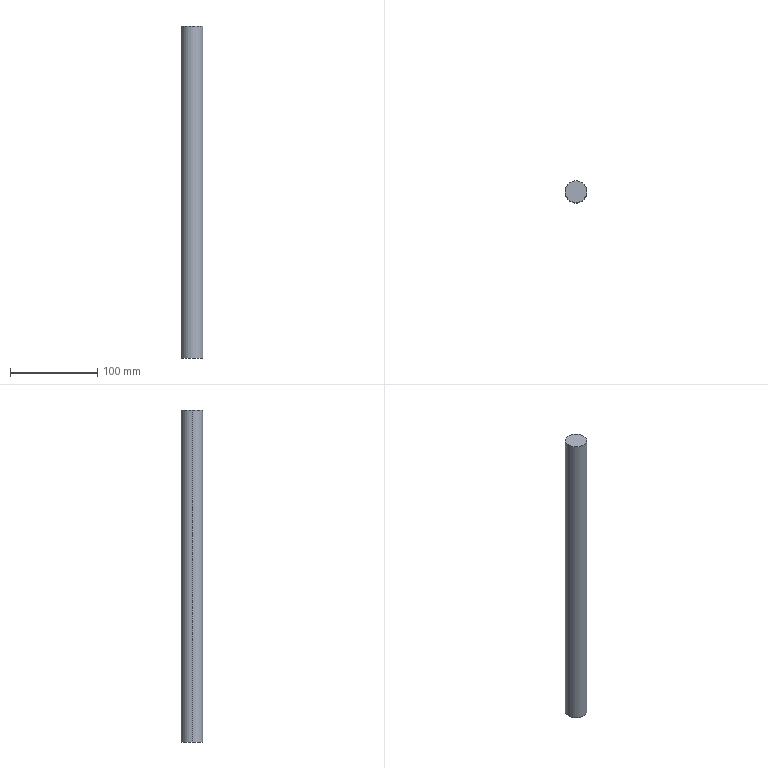Part | STEP file | 1 solid | 4 faces | box 25 x 25 x 380 mm | volume 186532 mm3 | cylinder 2 | plane 2 | commonest cylinder face diameters 25 x2
STEP:
#1=CARTESIAN_POINT('',(0.,0.,0.));
#2=DIRECTION('',(0.,0.,1.));
#3=DIRECTION('',(1.,0.,0.));
#4=AXIS2_PLACEMENT_3D('',#1,#2,#3);
#5=CARTESIAN_POINT('',(12.5,0.,190.));
#6=VERTEX_POINT('',#5);
#7=CARTESIAN_POINT('',(-12.5,0.,190.));
#8=VERTEX_POINT('',#7);
#9=CARTESIAN_POINT('',(0.,0.,190.));
#10=DIRECTION('',(0.,0.,1.));
#11=DIRECTION('',(1.,0.,0.));
#12=AXIS2_PLACEMENT_3D('',#9,#10,#11);
#13=CIRCLE('',#12,12.5);
#14=CARTESIAN_POINT('',(0.,0.,190.));
#15=DIRECTION('',(0.,0.,-1.));
#16=DIRECTION('',(-1.,0.,0.));
#17=AXIS2_PLACEMENT_3D('',#14,#15,#16);
#18=CYLINDRICAL_SURFACE('',#17,12.5);
#19=CARTESIAN_POINT('',(3.142,0.));
#20=DIRECTION('',(-1.,0.));
#21=VECTOR('',#20,1.);
#22=LINE('',#19,#21);
#23=(GEOMETRIC_REPRESENTATION_CONTEXT(2)PARAMETRIC_REPRESENTATION_CONTEXT()REPRESENTATION_CONTEXT('',''));
#24=DEFINITIONAL_REPRESENTATION('',(#22),#23);
#25=PCURVE('',#18,#24);
#26=CARTESIAN_POINT('',(0.,0.,190.));
#27=DIRECTION('',(0.,0.,1.));
#28=DIRECTION('',(1.,0.,0.));
#29=AXIS2_PLACEMENT_3D('',#26,#27,#28);
#30=PLANE('',#29);
#31=CARTESIAN_POINT('',(0.,0.));
#32=DIRECTION('',(1.,0.));
#33=AXIS2_PLACEMENT_2D('',#31,#32);
#34=CIRCLE('',#33,12.5);
#35=(GEOMETRIC_REPRESENTATION_CONTEXT(2)PARAMETRIC_REPRESENTATION_CONTEXT()REPRESENTATION_CONTEXT('',''));
#36=DEFINITIONAL_REPRESENTATION('',(#34),#35);
#37=PCURVE('',#30,#36);
#38=SURFACE_CURVE('',#13,(#25,#37),.PCURVE_S1.);
#39=EDGE_CURVE('',#6,#8,#38,.T.);
#40=ORIENTED_EDGE('',*,*,#39,.F.);
#41=CARTESIAN_POINT('',(12.5,0.,-190.));
#42=VERTEX_POINT('',#41);
#43=CARTESIAN_POINT('',(12.5,0.,190.));
#44=DIRECTION('',(0.,0.,-1.));
#45=VECTOR('',#44,1.);
#46=LINE('',#43,#45);
#47=CARTESIAN_POINT('',(3.142,0.));
#48=DIRECTION('',(0.,1.));
#49=VECTOR('',#48,1.);
#50=LINE('',#47,#49);
#51=(GEOMETRIC_REPRESENTATION_CONTEXT(2)PARAMETRIC_REPRESENTATION_CONTEXT()REPRESENTATION_CONTEXT('',''));
#52=DEFINITIONAL_REPRESENTATION('',(#50),#51);
#53=PCURVE('',#18,#52);
#54=CARTESIAN_POINT('',(0.,0.,190.));
#55=DIRECTION('',(0.,0.,-1.));
#56=DIRECTION('',(-1.,0.,0.));
#57=AXIS2_PLACEMENT_3D('',#54,#55,#56);
#58=CYLINDRICAL_SURFACE('',#57,12.5);
#59=CARTESIAN_POINT('',(3.142,0.));
#60=DIRECTION('',(0.,1.));
#61=VECTOR('',#60,1.);
#62=LINE('',#59,#61);
#63=(GEOMETRIC_REPRESENTATION_CONTEXT(2)PARAMETRIC_REPRESENTATION_CONTEXT()REPRESENTATION_CONTEXT('',''));
#64=DEFINITIONAL_REPRESENTATION('',(#62),#63);
#65=PCURVE('',#58,#64);
#66=SURFACE_CURVE('',#46,(#53,#65),.PCURVE_S1.);
#67=EDGE_CURVE('',#6,#42,#66,.T.);
#68=ORIENTED_EDGE('',*,*,#67,.T.);
#69=CARTESIAN_POINT('',(-12.5,0.,-190.));
#70=VERTEX_POINT('',#69);
#71=CARTESIAN_POINT('',(0.,0.,-190.));
#72=DIRECTION('',(0.,0.,1.));
#73=DIRECTION('',(1.,0.,0.));
#74=AXIS2_PLACEMENT_3D('',#71,#72,#73);
#75=CIRCLE('',#74,12.5);
#76=CARTESIAN_POINT('',(3.142,380.));
#77=DIRECTION('',(-1.,0.));
#78=VECTOR('',#77,1.);
#79=LINE('',#76,#78);
#80=(GEOMETRIC_REPRESENTATION_CONTEXT(2)PARAMETRIC_REPRESENTATION_CONTEXT()REPRESENTATION_CONTEXT('',''));
#81=DEFINITIONAL_REPRESENTATION('',(#79),#80);
#82=PCURVE('',#18,#81);
#83=CARTESIAN_POINT('',(0.,0.,-190.));
#84=DIRECTION('',(0.,0.,1.));
#85=DIRECTION('',(1.,0.,0.));
#86=AXIS2_PLACEMENT_3D('',#83,#84,#85);
#87=PLANE('',#86);
#88=CARTESIAN_POINT('',(0.,0.));
#89=DIRECTION('',(1.,0.));
#90=AXIS2_PLACEMENT_2D('',#88,#89);
#91=CIRCLE('',#90,12.5);
#92=(GEOMETRIC_REPRESENTATION_CONTEXT(2)PARAMETRIC_REPRESENTATION_CONTEXT()REPRESENTATION_CONTEXT('',''));
#93=DEFINITIONAL_REPRESENTATION('',(#91),#92);
#94=PCURVE('',#87,#93);
#95=SURFACE_CURVE('',#75,(#82,#94),.PCURVE_S1.);
#96=EDGE_CURVE('',#42,#70,#95,.T.);
#97=ORIENTED_EDGE('',*,*,#96,.T.);
#98=CARTESIAN_POINT('',(-12.5,0.,190.));
#99=DIRECTION('',(0.,0.,-1.));
#100=VECTOR('',#99,1.);
#101=LINE('',#98,#100);
#102=CARTESIAN_POINT('',(0.,0.));
#103=DIRECTION('',(0.,1.));
#104=VECTOR('',#103,1.);
#105=LINE('',#102,#104);
#106=(GEOMETRIC_REPRESENTATION_CONTEXT(2)PARAMETRIC_REPRESENTATION_CONTEXT()REPRESENTATION_CONTEXT('',''));
#107=DEFINITIONAL_REPRESENTATION('',(#105),#106);
#108=PCURVE('',#18,#107);
#109=CARTESIAN_POINT('',(6.283,0.));
#110=DIRECTION('',(0.,1.));
#111=VECTOR('',#110,1.);
#112=LINE('',#109,#111);
#113=(GEOMETRIC_REPRESENTATION_CONTEXT(2)PARAMETRIC_REPRESENTATION_CONTEXT()REPRESENTATION_CONTEXT('',''));
#114=DEFINITIONAL_REPRESENTATION('',(#112),#113);
#115=PCURVE('',#58,#114);
#116=SURFACE_CURVE('',#101,(#108,#115),.PCURVE_S1.);
#117=EDGE_CURVE('',#8,#70,#116,.T.);
#118=ORIENTED_EDGE('',*,*,#117,.F.);
#119=EDGE_LOOP('',(#40,#68,#97,#118));
#120=FACE_BOUND('',#119,.T.);
#121=ADVANCED_FACE('',(#120),#18,.T.);
#122=ORIENTED_EDGE('',*,*,#67,.F.);
#123=CARTESIAN_POINT('',(0.,0.,190.));
#124=DIRECTION('',(0.,0.,1.));
#125=DIRECTION('',(1.,0.,0.));
#126=AXIS2_PLACEMENT_3D('',#123,#124,#125);
#127=CIRCLE('',#126,12.5);
#128=CARTESIAN_POINT('',(9.425,0.));
#129=DIRECTION('',(-1.,0.));
#130=VECTOR('',#129,1.);
#131=LINE('',#128,#130);
#132=(GEOMETRIC_REPRESENTATION_CONTEXT(2)PARAMETRIC_REPRESENTATION_CONTEXT()REPRESENTATION_CONTEXT('',''));
#133=DEFINITIONAL_REPRESENTATION('',(#131),#132);
#134=PCURVE('',#58,#133);
#135=CARTESIAN_POINT('',(0.,0.));
#136=DIRECTION('',(1.,0.));
#137=AXIS2_PLACEMENT_2D('',#135,#136);
#138=CIRCLE('',#137,12.5);
#139=(GEOMETRIC_REPRESENTATION_CONTEXT(2)PARAMETRIC_REPRESENTATION_CONTEXT()REPRESENTATION_CONTEXT('',''));
#140=DEFINITIONAL_REPRESENTATION('',(#138),#139);
#141=PCURVE('',#30,#140);
#142=SURFACE_CURVE('',#127,(#134,#141),.PCURVE_S1.);
#143=EDGE_CURVE('',#8,#6,#142,.T.);
#144=ORIENTED_EDGE('',*,*,#143,.F.);
#145=ORIENTED_EDGE('',*,*,#117,.T.);
#146=CARTESIAN_POINT('',(0.,0.,-190.));
#147=DIRECTION('',(0.,0.,1.));
#148=DIRECTION('',(1.,0.,0.));
#149=AXIS2_PLACEMENT_3D('',#146,#147,#148);
#150=CIRCLE('',#149,12.5);
#151=CARTESIAN_POINT('',(9.425,380.));
#152=DIRECTION('',(-1.,0.));
#153=VECTOR('',#152,1.);
#154=LINE('',#151,#153);
#155=(GEOMETRIC_REPRESENTATION_CONTEXT(2)PARAMETRIC_REPRESENTATION_CONTEXT()REPRESENTATION_CONTEXT('',''));
#156=DEFINITIONAL_REPRESENTATION('',(#154),#155);
#157=PCURVE('',#58,#156);
#158=CARTESIAN_POINT('',(0.,0.));
#159=DIRECTION('',(1.,0.));
#160=AXIS2_PLACEMENT_2D('',#158,#159);
#161=CIRCLE('',#160,12.5);
#162=(GEOMETRIC_REPRESENTATION_CONTEXT(2)PARAMETRIC_REPRESENTATION_CONTEXT()REPRESENTATION_CONTEXT('',''));
#163=DEFINITIONAL_REPRESENTATION('',(#161),#162);
#164=PCURVE('',#87,#163);
#165=SURFACE_CURVE('',#150,(#157,#164),.PCURVE_S1.);
#166=EDGE_CURVE('',#70,#42,#165,.T.);
#167=ORIENTED_EDGE('',*,*,#166,.T.);
#168=EDGE_LOOP('',(#122,#144,#145,#167));
#169=FACE_BOUND('',#168,.T.);
#170=ADVANCED_FACE('',(#169),#58,.T.);
#171=ORIENTED_EDGE('',*,*,#143,.T.);
#172=ORIENTED_EDGE('',*,*,#39,.T.);
#173=EDGE_LOOP('',(#171,#172));
#174=FACE_BOUND('',#173,.T.);
#175=ADVANCED_FACE('',(#174),#30,.T.);
#176=ORIENTED_EDGE('',*,*,#166,.F.);
#177=ORIENTED_EDGE('',*,*,#96,.F.);
#178=EDGE_LOOP('',(#176,#177));
#179=FACE_BOUND('',#178,.T.);
#180=ADVANCED_FACE('',(#179),#87,.F.);
#181=CLOSED_SHELL('',(#121,#170,#175,#180));
#182=MANIFOLD_SOLID_BREP('',#181);
#183=(LENGTH_UNIT()NAMED_UNIT(*)SI_UNIT(.MILLI.,.METRE.));
#184=UNCERTAINTY_MEASURE_WITH_UNIT(LENGTH_MEASURE(0.0000001),#183,'','');
#185=(NAMED_UNIT(*)PLANE_ANGLE_UNIT()SI_UNIT($,.RADIAN.));
#186=(NAMED_UNIT(*)SI_UNIT($,.STERADIAN.)SOLID_ANGLE_UNIT());
#187=(GEOMETRIC_REPRESENTATION_CONTEXT(3)GLOBAL_UNCERTAINTY_ASSIGNED_CONTEXT((#184))GLOBAL_UNIT_ASSIGNED_CONTEXT((#183,#185,#186))REPRESENTATION_CONTEXT('',''));
#188=ADVANCED_BREP_SHAPE_REPRESENTATION('',(#4,#182),#187);